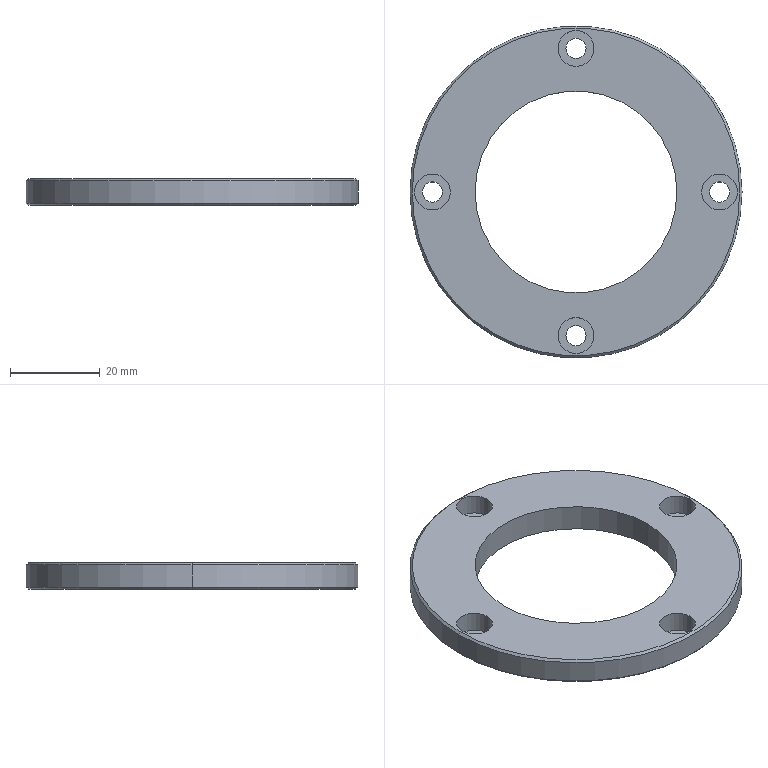Part | STEP file | 2088 Bag feed shaft end cap | 1 solid | 30 faces | box 74 x 74 x 6 mm | volume 15191 mm3 | cylinder 20 | plane 6 | cone 4 | commonest cylinder face diameters 4.5 x8 8 x8 45 x2 74 x2